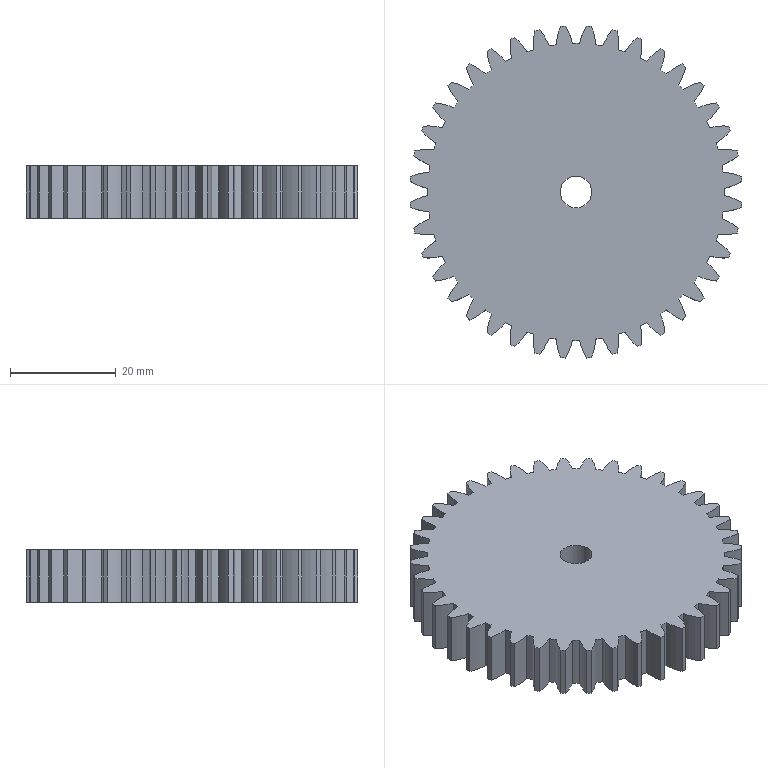Part | NX | features BREP 1 | 1 solid | 165 faces | box 62.872 x 62.872 x 10 mm | volume 27410 mm3 | cylinder 163 | plane 2 | commonest cylinder face diameters 24 x80 56.248 x41 63 x40 2.5 x1 6 x1